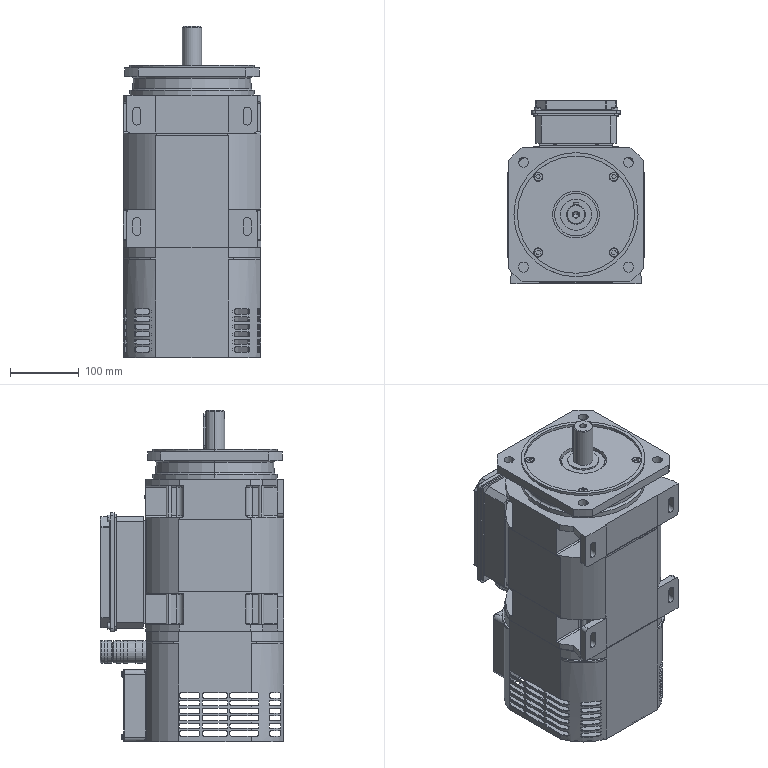Part | STEP file | motor_qs-100s-6_2-2600-360-87-b35-a | 6 solids | 1216 faces | box 200 x 266.5 x 480 mm | volume 10312452 mm3 | plane 579 | cylinder 541 | torus 64 | sphere 18 | cone 10 | spline 4 | commonest cylinder face diameters 4 x256 2 x68 8 x27 10 x14 12 x12 13 x12